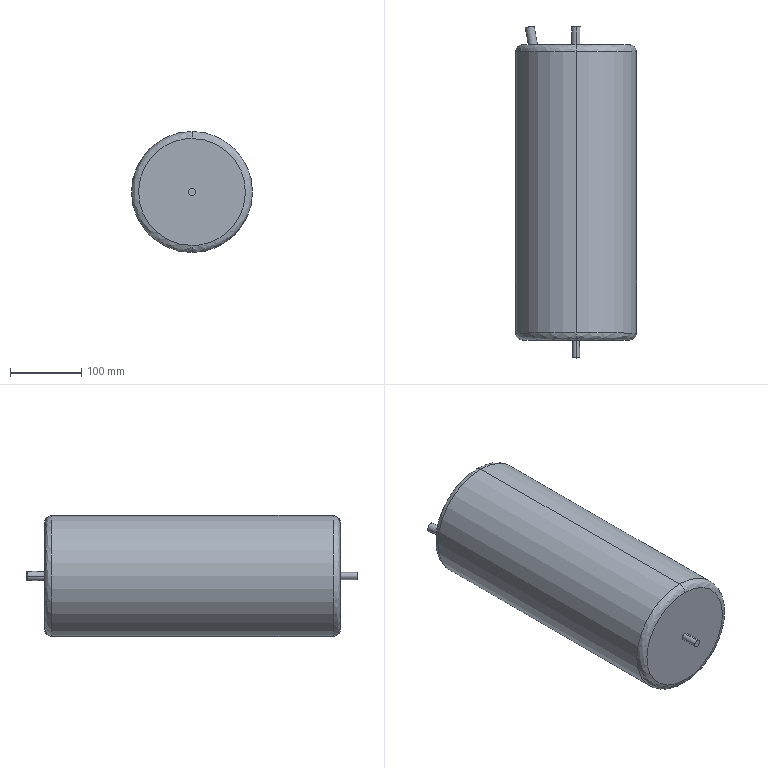Part | STEP file | TPLC-844-eight-litre receiver tank | 1 solid | 23 faces | box 170 x 466.103 x 170 mm | volume 9402386 mm3 | cylinder 12 | plane 7 | spline 4 | commonest cylinder face diameters 9.7 x4 12.7 x4 10 x2 170 x2